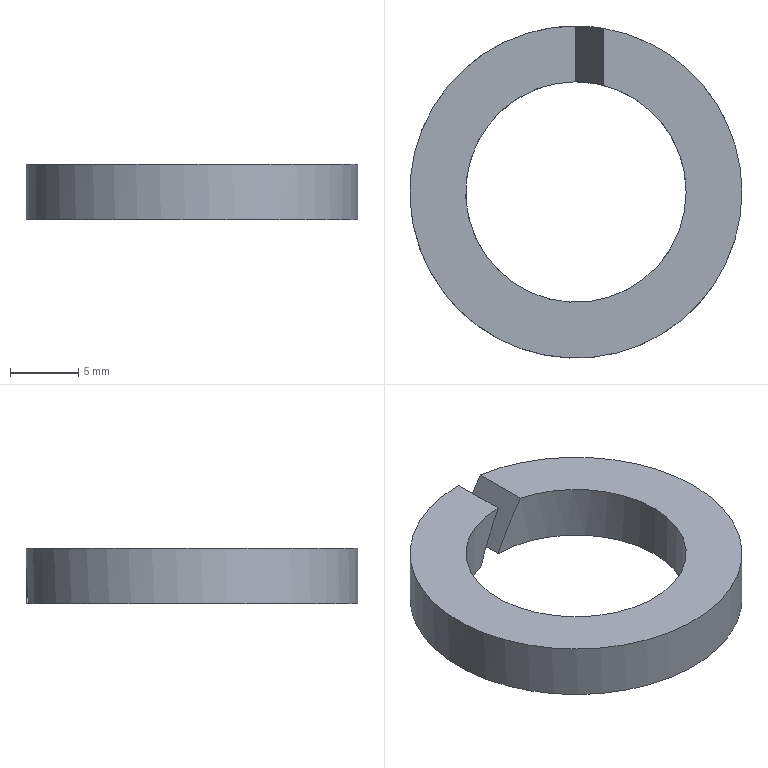Part | NX | features BREP 1 | 1 solid | 8 faces | box 24.4 x 24.4 x 4.1 mm | volume 1037 mm3 | plane 4 | cylinder 4 | commonest cylinder face diameters 16.2 x2 24.4 x2
STEP:
#1=CARTESIAN_POINT('',(-2.05,7.836,0.));
#2=VERTEX_POINT('',#1);
#3=CARTESIAN_POINT('',(8.1,0.,0.));
#4=VERTEX_POINT('',#3);
#5=CARTESIAN_POINT('',(0.,0.,0.));
#6=DIRECTION('',(0.,0.,1.));
#7=DIRECTION('',(-0.2531,0.9674,0.));
#8=AXIS2_PLACEMENT_3D('',#5,#6,#7);
#9=CIRCLE('',#8,8.1);
#10=EDGE_CURVE('',#2,#4,#9,.T.);
#11=ORIENTED_EDGE('',*,*,#10,.T.);
#12=CARTESIAN_POINT('',(0.,8.1,0.));
#13=VERTEX_POINT('',#12);
#14=CARTESIAN_POINT('',(0.,0.,0.));
#15=DIRECTION('',(0.,0.,-1.));
#16=DIRECTION('',(0.,1.,0.));
#17=AXIS2_PLACEMENT_3D('',#14,#15,#16);
#18=CIRCLE('',#17,8.1);
#19=EDGE_CURVE('',#13,#4,#18,.T.);
#20=ORIENTED_EDGE('',*,*,#19,.F.);
#21=CARTESIAN_POINT('',(0.,12.2,0.));
#22=VERTEX_POINT('',#21);
#23=CARTESIAN_POINT('',(0.,8.1,0.));
#24=DIRECTION('',(0.,1.,0.));
#25=VECTOR('',#24,1000.);
#26=LINE('',#23,#25);
#27=EDGE_CURVE('',#13,#22,#26,.T.);
#28=ORIENTED_EDGE('',*,*,#27,.T.);
#29=CARTESIAN_POINT('',(12.2,0.,0.));
#30=VERTEX_POINT('',#29);
#31=CARTESIAN_POINT('',(0.,0.,0.));
#32=DIRECTION('',(0.,0.,1.));
#33=DIRECTION('',(1.,0.,0.));
#34=AXIS2_PLACEMENT_3D('',#31,#32,#33);
#35=CIRCLE('',#34,12.2);
#36=EDGE_CURVE('',#30,#22,#35,.T.);
#37=ORIENTED_EDGE('',*,*,#36,.F.);
#38=CARTESIAN_POINT('',(-2.05,12.027,0.));
#39=VERTEX_POINT('',#38);
#40=CARTESIAN_POINT('',(0.,0.,0.));
#41=DIRECTION('',(0.,0.,-1.));
#42=DIRECTION('',(1.,0.,0.));
#43=AXIS2_PLACEMENT_3D('',#40,#41,#42);
#44=CIRCLE('',#43,12.2);
#45=EDGE_CURVE('',#30,#39,#44,.T.);
#46=ORIENTED_EDGE('',*,*,#45,.T.);
#47=CARTESIAN_POINT('',(-2.05,7.836,0.));
#48=DIRECTION('',(0.,1.,0.));
#49=VECTOR('',#48,1000.);
#50=LINE('',#47,#49);
#51=EDGE_CURVE('',#2,#39,#50,.T.);
#52=ORIENTED_EDGE('',*,*,#51,.F.);
#53=EDGE_LOOP('',(#11,#20,#28,#37,#46,#52));
#54=FACE_BOUND('',#53,.T.);
#55=CARTESIAN_POINT('',(0.,0.,0.));
#56=DIRECTION('',(0.,0.,1.));
#57=DIRECTION('',(-1.,0.,0.));
#58=AXIS2_PLACEMENT_3D('',#55,#56,#57);
#59=PLANE('',#58);
#60=ADVANCED_FACE('',(#54),#59,.F.);
#61=ORIENTED_EDGE('',*,*,#51,.T.);
#62=CARTESIAN_POINT('',(0.,12.2,4.1));
#63=VERTEX_POINT('',#62);
#64=CARTESIAN_POINT('',(0.,0.,4.1));
#65=DIRECTION('',(-0.8944,0.,0.4472));
#66=DIRECTION('',(0.4472,0.,0.8944));
#67=AXIS2_PLACEMENT_3D('',#64,#65,#66);
#68=ELLIPSE('',#67,27.28,12.2);
#69=EDGE_CURVE('',#63,#39,#68,.T.);
#70=ORIENTED_EDGE('',*,*,#69,.F.);
#71=CARTESIAN_POINT('',(0.,8.1,4.1));
#72=VERTEX_POINT('',#71);
#73=CARTESIAN_POINT('',(0.,8.1,4.1));
#74=DIRECTION('',(0.,1.,0.));
#75=VECTOR('',#74,1000.);
#76=LINE('',#73,#75);
#77=EDGE_CURVE('',#72,#63,#76,.T.);
#78=ORIENTED_EDGE('',*,*,#77,.F.);
#79=CARTESIAN_POINT('',(0.,0.,4.1));
#80=DIRECTION('',(-0.8944,0.,0.4472));
#81=DIRECTION('',(0.4472,0.,0.8944));
#82=AXIS2_PLACEMENT_3D('',#79,#80,#81);
#83=ELLIPSE('',#82,18.112,8.1);
#84=EDGE_CURVE('',#72,#2,#83,.T.);
#85=ORIENTED_EDGE('',*,*,#84,.T.);
#86=EDGE_LOOP('',(#61,#70,#78,#85));
#87=FACE_BOUND('',#86,.T.);
#88=CARTESIAN_POINT('',(-2.05,0.,0.));
#89=DIRECTION('',(-0.8944,0.,0.4472));
#90=DIRECTION('',(-0.4472,0.,-0.8944));
#91=AXIS2_PLACEMENT_3D('',#88,#89,#90);
#92=PLANE('',#91);
#93=ADVANCED_FACE('',(#87),#92,.F.);
#94=CARTESIAN_POINT('',(8.1,0.,4.1));
#95=VERTEX_POINT('',#94);
#96=CARTESIAN_POINT('',(8.1,0.,0.));
#97=DIRECTION('',(0.,0.,1.));
#98=VECTOR('',#97,1000.);
#99=LINE('',#96,#98);
#100=EDGE_CURVE('',#4,#95,#99,.T.);
#101=ORIENTED_EDGE('',*,*,#100,.F.);
#102=ORIENTED_EDGE('',*,*,#10,.F.);
#103=ORIENTED_EDGE('',*,*,#84,.F.);
#104=CARTESIAN_POINT('',(0.,0.,4.1));
#105=DIRECTION('',(0.,0.,-1.));
#106=DIRECTION('',(1.,0.,0.));
#107=AXIS2_PLACEMENT_3D('',#104,#105,#106);
#108=CIRCLE('',#107,8.1);
#109=EDGE_CURVE('',#95,#72,#108,.T.);
#110=ORIENTED_EDGE('',*,*,#109,.F.);
#111=EDGE_LOOP('',(#101,#102,#103,#110));
#112=FACE_BOUND('',#111,.T.);
#113=CARTESIAN_POINT('',(0.,0.,0.));
#114=DIRECTION('',(0.,0.,1.));
#115=DIRECTION('',(-1.,0.,0.));
#116=AXIS2_PLACEMENT_3D('',#113,#114,#115);
#117=CYLINDRICAL_SURFACE('',#116,8.1);
#118=ADVANCED_FACE('',(#112),#117,.F.);
#119=CARTESIAN_POINT('',(12.2,0.,4.1));
#120=VERTEX_POINT('',#119);
#121=CARTESIAN_POINT('',(0.,0.,4.1));
#122=DIRECTION('',(0.,0.,1.));
#123=DIRECTION('',(0.,1.,0.));
#124=AXIS2_PLACEMENT_3D('',#121,#122,#123);
#125=CIRCLE('',#124,12.2);
#126=EDGE_CURVE('',#63,#120,#125,.T.);
#127=ORIENTED_EDGE('',*,*,#126,.T.);
#128=CARTESIAN_POINT('',(2.05,12.027,4.1));
#129=VERTEX_POINT('',#128);
#130=CARTESIAN_POINT('',(0.,0.,4.1));
#131=DIRECTION('',(0.,0.,1.));
#132=DIRECTION('',(1.,0.,0.));
#133=AXIS2_PLACEMENT_3D('',#130,#131,#132);
#134=CIRCLE('',#133,12.2);
#135=EDGE_CURVE('',#120,#129,#134,.T.);
#136=ORIENTED_EDGE('',*,*,#135,.T.);
#137=CARTESIAN_POINT('',(2.05,7.836,4.1));
#138=VERTEX_POINT('',#137);
#139=CARTESIAN_POINT('',(2.05,7.836,4.1));
#140=DIRECTION('',(0.,1.,0.));
#141=VECTOR('',#140,1000.);
#142=LINE('',#139,#141);
#143=EDGE_CURVE('',#138,#129,#142,.T.);
#144=ORIENTED_EDGE('',*,*,#143,.F.);
#145=CARTESIAN_POINT('',(0.,0.,4.1));
#146=DIRECTION('',(0.,0.,-1.));
#147=DIRECTION('',(0.2531,0.9674,0.));
#148=AXIS2_PLACEMENT_3D('',#145,#146,#147);
#149=CIRCLE('',#148,8.1);
#150=EDGE_CURVE('',#138,#95,#149,.T.);
#151=ORIENTED_EDGE('',*,*,#150,.T.);
#152=ORIENTED_EDGE('',*,*,#109,.T.);
#153=ORIENTED_EDGE('',*,*,#77,.T.);
#154=EDGE_LOOP('',(#127,#136,#144,#151,#152,#153));
#155=FACE_BOUND('',#154,.T.);
#156=CARTESIAN_POINT('',(0.,0.,4.1));
#157=DIRECTION('',(0.,0.,1.));
#158=DIRECTION('',(-1.,0.,0.));
#159=AXIS2_PLACEMENT_3D('',#156,#157,#158);
#160=PLANE('',#159);
#161=ADVANCED_FACE('',(#155),#160,.T.);
#162=ORIENTED_EDGE('',*,*,#19,.T.);
#163=ORIENTED_EDGE('',*,*,#100,.T.);
#164=ORIENTED_EDGE('',*,*,#150,.F.);
#165=CARTESIAN_POINT('',(0.,0.,0.));
#166=DIRECTION('',(0.8944,0.,-0.4472));
#167=DIRECTION('',(0.4472,0.,0.8944));
#168=AXIS2_PLACEMENT_3D('',#165,#166,#167);
#169=ELLIPSE('',#168,18.112,8.1);
#170=EDGE_CURVE('',#138,#13,#169,.F.);
#171=ORIENTED_EDGE('',*,*,#170,.T.);
#172=EDGE_LOOP('',(#162,#163,#164,#171));
#173=FACE_BOUND('',#172,.T.);
#174=CARTESIAN_POINT('',(0.,0.,0.));
#175=DIRECTION('',(0.,0.,1.));
#176=DIRECTION('',(-1.,0.,0.));
#177=AXIS2_PLACEMENT_3D('',#174,#175,#176);
#178=CYLINDRICAL_SURFACE('',#177,8.1);
#179=ADVANCED_FACE('',(#173),#178,.F.);
#180=ORIENTED_EDGE('',*,*,#27,.F.);
#181=ORIENTED_EDGE('',*,*,#170,.F.);
#182=ORIENTED_EDGE('',*,*,#143,.T.);
#183=CARTESIAN_POINT('',(0.,0.,0.));
#184=DIRECTION('',(0.8944,0.,-0.4472));
#185=DIRECTION('',(0.4472,0.,0.8944));
#186=AXIS2_PLACEMENT_3D('',#183,#184,#185);
#187=ELLIPSE('',#186,27.28,12.2);
#188=EDGE_CURVE('',#129,#22,#187,.F.);
#189=ORIENTED_EDGE('',*,*,#188,.T.);
#190=EDGE_LOOP('',(#180,#181,#182,#189));
#191=FACE_BOUND('',#190,.T.);
#192=CARTESIAN_POINT('',(2.05,0.,4.1));
#193=DIRECTION('',(0.8944,0.,-0.4472));
#194=DIRECTION('',(0.4472,0.,0.8944));
#195=AXIS2_PLACEMENT_3D('',#192,#193,#194);
#196=PLANE('',#195);
#197=ADVANCED_FACE('',(#191),#196,.F.);
#198=ORIENTED_EDGE('',*,*,#135,.F.);
#199=CARTESIAN_POINT('',(12.2,0.,0.));
#200=DIRECTION('',(0.,0.,1.));
#201=VECTOR('',#200,1000.);
#202=LINE('',#199,#201);
#203=EDGE_CURVE('',#30,#120,#202,.T.);
#204=ORIENTED_EDGE('',*,*,#203,.F.);
#205=ORIENTED_EDGE('',*,*,#36,.T.);
#206=ORIENTED_EDGE('',*,*,#188,.F.);
#207=EDGE_LOOP('',(#198,#204,#205,#206));
#208=FACE_BOUND('',#207,.T.);
#209=CARTESIAN_POINT('',(0.,0.,0.));
#210=DIRECTION('',(0.,0.,1.));
#211=DIRECTION('',(-1.,0.,0.));
#212=AXIS2_PLACEMENT_3D('',#209,#210,#211);
#213=CYLINDRICAL_SURFACE('',#212,12.2);
#214=ADVANCED_FACE('',(#208),#213,.T.);
#215=ORIENTED_EDGE('',*,*,#203,.T.);
#216=ORIENTED_EDGE('',*,*,#126,.F.);
#217=ORIENTED_EDGE('',*,*,#69,.T.);
#218=ORIENTED_EDGE('',*,*,#45,.F.);
#219=EDGE_LOOP('',(#215,#216,#217,#218));
#220=FACE_BOUND('',#219,.T.);
#221=CARTESIAN_POINT('',(0.,0.,0.));
#222=DIRECTION('',(0.,0.,1.));
#223=DIRECTION('',(-1.,0.,0.));
#224=AXIS2_PLACEMENT_3D('',#221,#222,#223);
#225=CYLINDRICAL_SURFACE('',#224,12.2);
#226=ADVANCED_FACE('',(#220),#225,.T.);
#227=CLOSED_SHELL('',(#60,#93,#118,#161,#179,#197,#214,#226));
#228=MANIFOLD_SOLID_BREP('',#227);
#229=(LENGTH_UNIT()NAMED_UNIT(*)SI_UNIT(.MILLI.,.METRE.));
#230=UNCERTAINTY_MEASURE_WITH_UNIT(LENGTH_MEASURE(0.00001),#229,'','');
#231=(NAMED_UNIT(*)PLANE_ANGLE_UNIT()SI_UNIT($,.RADIAN.));
#232=(NAMED_UNIT(*)SI_UNIT($,.STERADIAN.)SOLID_ANGLE_UNIT());
#233=(GEOMETRIC_REPRESENTATION_CONTEXT(3)GLOBAL_UNCERTAINTY_ASSIGNED_CONTEXT((#230))GLOBAL_UNIT_ASSIGNED_CONTEXT((#229,#231,#232))REPRESENTATION_CONTEXT('',''));
#234=ADVANCED_BREP_SHAPE_REPRESENTATION('',(#228),#233);